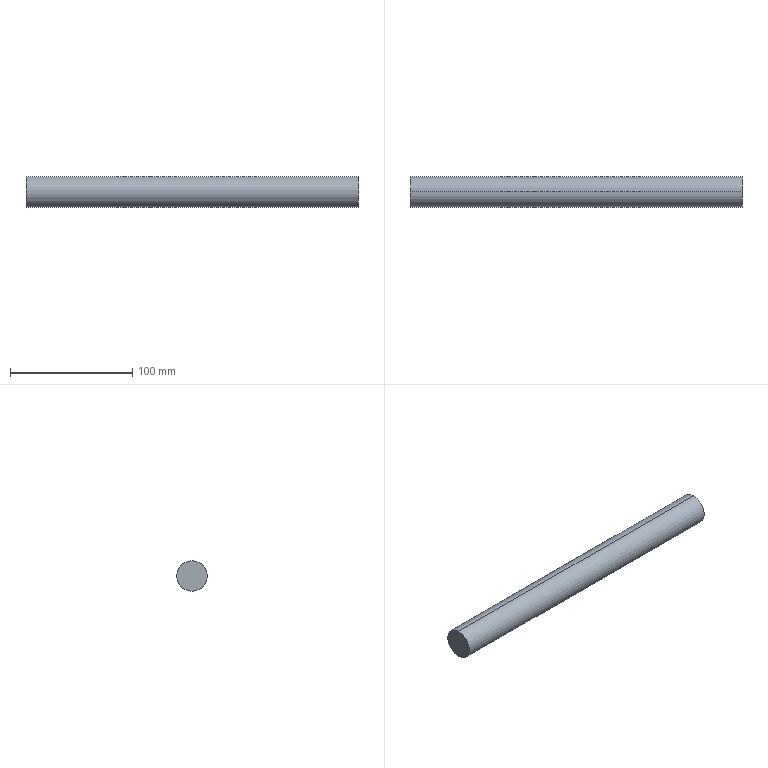Part | SolidWorks | features Extrusion 1 | 1 solid | 4 faces | box 272 x 25 x 25 mm | volume 133518 mm3 | cylinder 2 | plane 2 | commonest cylinder face diameters 25 x2
STEP:
#1=CARTESIAN_POINT('',(136.,0.,-12.5));
#2=VERTEX_POINT('',#1);
#3=CARTESIAN_POINT('',(136.,0.,12.5));
#4=VERTEX_POINT('',#3);
#5=CARTESIAN_POINT('',(136.,0.,0.));
#6=DIRECTION('',(1.,0.,0.));
#7=DIRECTION('',(0.,0.,-1.));
#8=AXIS2_PLACEMENT_3D('',#5,#6,#7);
#9=CIRCLE('',#8,12.5);
#10=EDGE_CURVE('',#2,#4,#9,.T.);
#11=ORIENTED_EDGE('',*,*,#10,.F.);
#12=CARTESIAN_POINT('',(-136.,0.,-12.5));
#13=VERTEX_POINT('',#12);
#14=CARTESIAN_POINT('',(136.,0.,-12.5));
#15=DIRECTION('',(-1.,0.,0.));
#16=VECTOR('',#15,1000.);
#17=LINE('',#14,#16);
#18=EDGE_CURVE('',#2,#13,#17,.T.);
#19=ORIENTED_EDGE('',*,*,#18,.T.);
#20=CARTESIAN_POINT('',(-136.,0.,12.5));
#21=VERTEX_POINT('',#20);
#22=CARTESIAN_POINT('',(-136.,0.,0.));
#23=DIRECTION('',(1.,0.,0.));
#24=DIRECTION('',(0.,0.,-1.));
#25=AXIS2_PLACEMENT_3D('',#22,#23,#24);
#26=CIRCLE('',#25,12.5);
#27=EDGE_CURVE('',#13,#21,#26,.T.);
#28=ORIENTED_EDGE('',*,*,#27,.T.);
#29=CARTESIAN_POINT('',(136.,0.,12.5));
#30=DIRECTION('',(-1.,0.,0.));
#31=VECTOR('',#30,1000.);
#32=LINE('',#29,#31);
#33=EDGE_CURVE('',#4,#21,#32,.T.);
#34=ORIENTED_EDGE('',*,*,#33,.F.);
#35=EDGE_LOOP('',(#11,#19,#28,#34));
#36=FACE_OUTER_BOUND('',#35,.T.);
#37=CARTESIAN_POINT('',(136.,0.,0.));
#38=DIRECTION('',(-1.,0.,0.));
#39=DIRECTION('',(0.,0.,1.));
#40=AXIS2_PLACEMENT_3D('',#37,#38,#39);
#41=CYLINDRICAL_SURFACE('',#40,12.5);
#42=ADVANCED_FACE('',(#36),#41,.T.);
#43=ORIENTED_EDGE('',*,*,#18,.F.);
#44=CARTESIAN_POINT('',(136.,0.,0.));
#45=DIRECTION('',(1.,0.,0.));
#46=DIRECTION('',(0.,0.,-1.));
#47=AXIS2_PLACEMENT_3D('',#44,#45,#46);
#48=CIRCLE('',#47,12.5);
#49=EDGE_CURVE('',#4,#2,#48,.T.);
#50=ORIENTED_EDGE('',*,*,#49,.F.);
#51=ORIENTED_EDGE('',*,*,#33,.T.);
#52=CARTESIAN_POINT('',(-136.,0.,0.));
#53=DIRECTION('',(1.,0.,0.));
#54=DIRECTION('',(0.,0.,-1.));
#55=AXIS2_PLACEMENT_3D('',#52,#53,#54);
#56=CIRCLE('',#55,12.5);
#57=EDGE_CURVE('',#21,#13,#56,.T.);
#58=ORIENTED_EDGE('',*,*,#57,.T.);
#59=EDGE_LOOP('',(#43,#50,#51,#58));
#60=FACE_OUTER_BOUND('',#59,.T.);
#61=CARTESIAN_POINT('',(136.,0.,0.));
#62=DIRECTION('',(-1.,0.,0.));
#63=DIRECTION('',(0.,0.,1.));
#64=AXIS2_PLACEMENT_3D('',#61,#62,#63);
#65=CYLINDRICAL_SURFACE('',#64,12.5);
#66=ADVANCED_FACE('',(#60),#65,.T.);
#67=ORIENTED_EDGE('',*,*,#49,.T.);
#68=ORIENTED_EDGE('',*,*,#10,.T.);
#69=EDGE_LOOP('',(#67,#68));
#70=FACE_OUTER_BOUND('',#69,.T.);
#71=CARTESIAN_POINT('',(136.,0.,0.));
#72=DIRECTION('',(1.,0.,0.));
#73=DIRECTION('',(0.,0.,-1.));
#74=AXIS2_PLACEMENT_3D('',#71,#72,#73);
#75=PLANE('',#74);
#76=ADVANCED_FACE('',(#70),#75,.T.);
#77=ORIENTED_EDGE('',*,*,#57,.F.);
#78=ORIENTED_EDGE('',*,*,#27,.F.);
#79=EDGE_LOOP('',(#77,#78));
#80=FACE_OUTER_BOUND('',#79,.T.);
#81=CARTESIAN_POINT('',(-136.,0.,0.));
#82=DIRECTION('',(1.,0.,0.));
#83=DIRECTION('',(0.,0.,-1.));
#84=AXIS2_PLACEMENT_3D('',#81,#82,#83);
#85=PLANE('',#84);
#86=ADVANCED_FACE('',(#80),#85,.F.);
#87=CLOSED_SHELL('',(#42,#66,#76,#86));
#88=MANIFOLD_SOLID_BREP('',#87);
#89=CARTESIAN_POINT('',(0.,0.,0.));
#90=DIRECTION('',(0.,0.,1.));
#91=DIRECTION('',(1.,0.,0.));
#92=AXIS2_PLACEMENT_3D('',#89,#90,#91);
#93=(LENGTH_UNIT()NAMED_UNIT(*)SI_UNIT(.MILLI.,.METRE.));
#94=UNCERTAINTY_MEASURE_WITH_UNIT(LENGTH_MEASURE(0.00001),#93,'','');
#95=(NAMED_UNIT(*)PLANE_ANGLE_UNIT()SI_UNIT($,.RADIAN.));
#96=(NAMED_UNIT(*)SI_UNIT($,.STERADIAN.)SOLID_ANGLE_UNIT());
#97=(GEOMETRIC_REPRESENTATION_CONTEXT(3)GLOBAL_UNCERTAINTY_ASSIGNED_CONTEXT((#94))GLOBAL_UNIT_ASSIGNED_CONTEXT((#93,#95,#96))REPRESENTATION_CONTEXT('',''));
#98=ADVANCED_BREP_SHAPE_REPRESENTATION('',(#88,#92),#97);